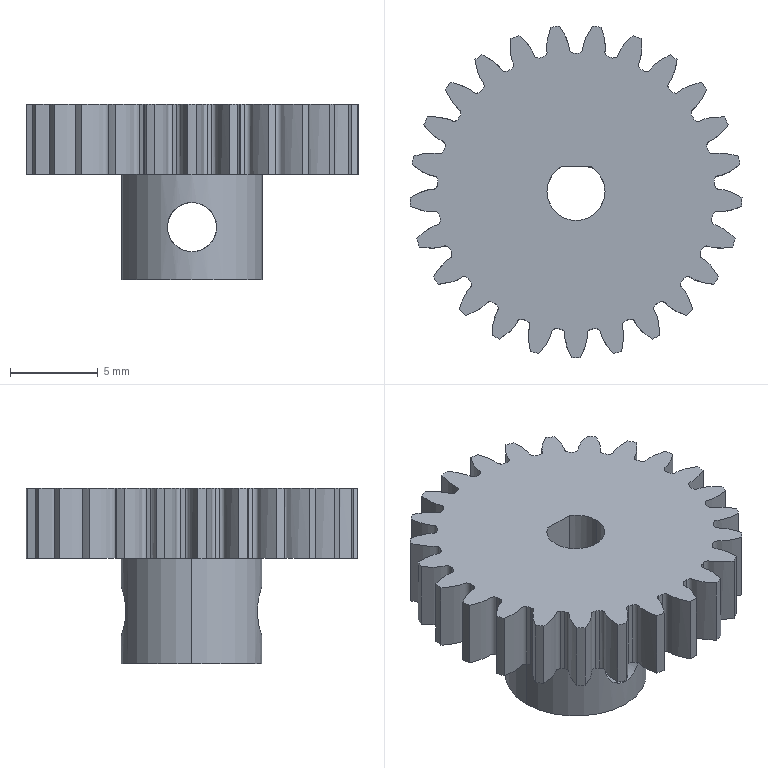Part | SolidWorks | features ICE 7, CirPattern 1, Extrusion 1, RefAxis 1 | 1 solid | 113 faces | box 18.888 x 18.854 x 10 mm | volume 1132 mm3 | cylinder 58 | spline 50 | plane 5 | commonest cylinder face diameters 15.75 x25 18.9 x25 2.8 x4 3.3 x2 8 x2